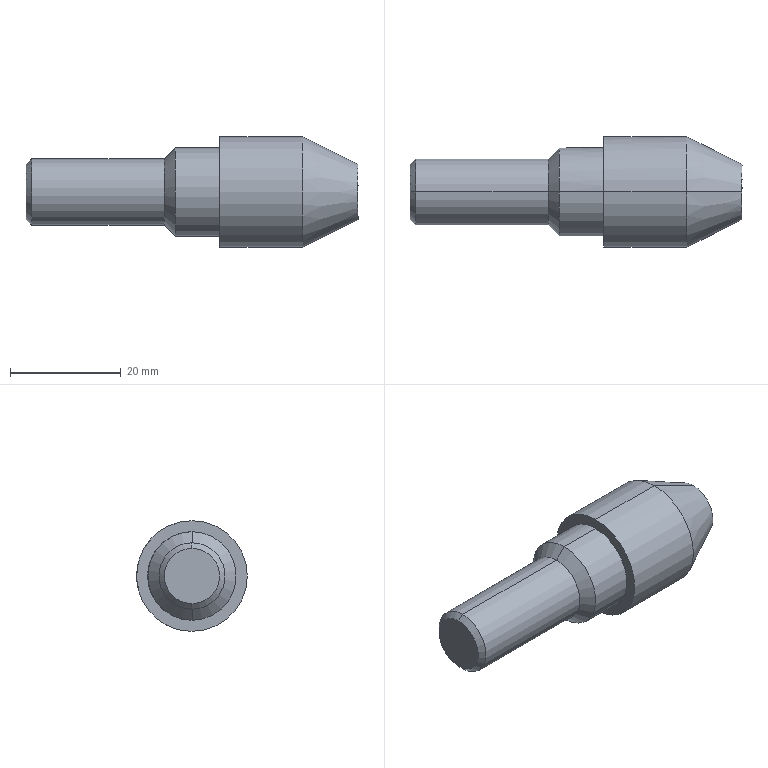Part | STEP file | Positioning_id698_x_t | 1 solid | 15 faces | box 60 x 20 x 20 mm | volume 11273 mm3 | cone 6 | cylinder 6 | plane 3 | commonest cylinder face diameters 12 x2 16 x2 20 x2
STEP:
#1=CARTESIAN_POINT('',(0.,0.,0.));
#2=DIRECTION('',(0.,0.,1.));
#3=DIRECTION('',(1.,0.,0.));
#4=AXIS2_PLACEMENT_3D('',#1,#2,#3);
#5=CARTESIAN_POINT('',(-988.002,780.,192.466));
#6=VERTEX_POINT('',#5);
#7=CARTESIAN_POINT('',(-998.002,780.,187.466));
#8=VERTEX_POINT('',#7);
#9=CARTESIAN_POINT('',(-988.002,780.,192.466));
#10=DIRECTION('',(-0.8944,0.,-0.4472));
#11=VECTOR('',#10,1.);
#12=LINE('',#9,#11);
#13=CARTESIAN_POINT('',(-998.002,780.,197.466));
#14=DIRECTION('',(-1.,0.,0.));
#15=DIRECTION('',(0.,0.,-1.));
#16=AXIS2_PLACEMENT_3D('',#13,#14,#15);
#17=CONICAL_SURFACE('',#16,10.,0.4636);
#18=CARTESIAN_POINT('',(0.,-10.));
#19=DIRECTION('',(0.,1.));
#20=VECTOR('',#19,1.);
#21=LINE('',#18,#20);
#22=(GEOMETRIC_REPRESENTATION_CONTEXT(2)PARAMETRIC_REPRESENTATION_CONTEXT()REPRESENTATION_CONTEXT('',''));
#23=DEFINITIONAL_REPRESENTATION('',(#21),#22);
#24=PCURVE('',#17,#23);
#25=CARTESIAN_POINT('',(-998.002,780.,197.466));
#26=DIRECTION('',(-1.,0.,0.));
#27=DIRECTION('',(0.,0.,-1.));
#28=AXIS2_PLACEMENT_3D('',#25,#26,#27);
#29=CONICAL_SURFACE('',#28,10.,0.4636);
#30=CARTESIAN_POINT('',(6.283,-10.));
#31=DIRECTION('',(0.,1.));
#32=VECTOR('',#31,1.);
#33=LINE('',#30,#32);
#34=(GEOMETRIC_REPRESENTATION_CONTEXT(2)PARAMETRIC_REPRESENTATION_CONTEXT()REPRESENTATION_CONTEXT('',''));
#35=DEFINITIONAL_REPRESENTATION('',(#33),#34);
#36=PCURVE('',#29,#35);
#37=SURFACE_CURVE('',#12,(#24,#36),.PCURVE_S1.);
#38=EDGE_CURVE('',#6,#8,#37,.T.);
#39=ORIENTED_EDGE('',*,*,#38,.F.);
#40=CARTESIAN_POINT('',(-988.002,780.,202.466));
#41=VERTEX_POINT('',#40);
#42=CARTESIAN_POINT('',(-988.002,780.,197.466));
#43=DIRECTION('',(-1.,0.,0.));
#44=DIRECTION('',(0.,-1.,0.));
#45=AXIS2_PLACEMENT_3D('',#42,#43,#44);
#46=CIRCLE('',#45,5.);
#47=CARTESIAN_POINT('',(-4.712,-10.));
#48=DIRECTION('',(1.,0.));
#49=VECTOR('',#48,1.);
#50=LINE('',#47,#49);
#51=(GEOMETRIC_REPRESENTATION_CONTEXT(2)PARAMETRIC_REPRESENTATION_CONTEXT()REPRESENTATION_CONTEXT('',''));
#52=DEFINITIONAL_REPRESENTATION('',(#50),#51);
#53=PCURVE('',#17,#52);
#54=CARTESIAN_POINT('',(-988.002,780.,197.466));
#55=DIRECTION('',(1.,0.,0.));
#56=DIRECTION('',(0.,0.,1.));
#57=AXIS2_PLACEMENT_3D('',#54,#55,#56);
#58=PLANE('',#57);
#59=CARTESIAN_POINT('',(0.,5.));
#60=CARTESIAN_POINT('',(8.66,5.));
#61=CARTESIAN_POINT('',(4.33,-2.5));
#62=CARTESIAN_POINT('',(0.,-10.));
#63=CARTESIAN_POINT('',(-4.33,-2.5));
#64=CARTESIAN_POINT('',(-8.66,5.));
#65=CARTESIAN_POINT('',(0.,5.));
#66=(BOUNDED_CURVE()B_SPLINE_CURVE(2,(#59,#60,#61,#62,#63,#64,#65),.UNSPECIFIED.,.T.,.F.)B_SPLINE_CURVE_WITH_KNOTS((1,2,2,2,2,1),(-2.094,0.,2.094,4.189,6.283,8.378),.UNSPECIFIED.)CURVE()GEOMETRIC_REPRESENTATION_ITEM()RATIONAL_B_SPLINE_CURVE((1.,0.5,1.,0.5,1.,0.5,1.))REPRESENTATION_ITEM(''));
#67=(GEOMETRIC_REPRESENTATION_CONTEXT(2)PARAMETRIC_REPRESENTATION_CONTEXT()REPRESENTATION_CONTEXT('',''));
#68=DEFINITIONAL_REPRESENTATION('',(#66),#67);
#69=PCURVE('',#58,#68);
#70=SURFACE_CURVE('',#46,(#53,#69),.PCURVE_S1.);
#71=EDGE_CURVE('',#6,#41,#70,.T.);
#72=ORIENTED_EDGE('',*,*,#71,.T.);
#73=CARTESIAN_POINT('',(-998.002,780.,207.466));
#74=VERTEX_POINT('',#73);
#75=CARTESIAN_POINT('',(-988.002,780.,202.466));
#76=DIRECTION('',(0.8944,0.,-0.4472));
#77=VECTOR('',#76,1.);
#78=LINE('',#75,#77);
#79=CARTESIAN_POINT('',(3.142,-10.));
#80=DIRECTION('',(0.,-1.));
#81=VECTOR('',#80,1.);
#82=LINE('',#79,#81);
#83=(GEOMETRIC_REPRESENTATION_CONTEXT(2)PARAMETRIC_REPRESENTATION_CONTEXT()REPRESENTATION_CONTEXT('',''));
#84=DEFINITIONAL_REPRESENTATION('',(#82),#83);
#85=PCURVE('',#17,#84);
#86=CARTESIAN_POINT('',(3.142,-10.));
#87=DIRECTION('',(0.,-1.));
#88=VECTOR('',#87,1.);
#89=LINE('',#86,#88);
#90=(GEOMETRIC_REPRESENTATION_CONTEXT(2)PARAMETRIC_REPRESENTATION_CONTEXT()REPRESENTATION_CONTEXT('',''));
#91=DEFINITIONAL_REPRESENTATION('',(#89),#90);
#92=PCURVE('',#29,#91);
#93=SURFACE_CURVE('',#78,(#85,#92),.PCURVE_S1.);
#94=EDGE_CURVE('',#74,#41,#93,.T.);
#95=ORIENTED_EDGE('',*,*,#94,.F.);
#96=CARTESIAN_POINT('',(-998.002,780.,197.466));
#97=DIRECTION('',(-1.,0.,0.));
#98=DIRECTION('',(0.,0.,-1.));
#99=AXIS2_PLACEMENT_3D('',#96,#97,#98);
#100=CIRCLE('',#99,10.);
#101=CARTESIAN_POINT('',(0.,0.));
#102=DIRECTION('',(1.,0.));
#103=VECTOR('',#102,1.);
#104=LINE('',#101,#103);
#105=(GEOMETRIC_REPRESENTATION_CONTEXT(2)PARAMETRIC_REPRESENTATION_CONTEXT()REPRESENTATION_CONTEXT('',''));
#106=DEFINITIONAL_REPRESENTATION('',(#104),#105);
#107=PCURVE('',#17,#106);
#108=CARTESIAN_POINT('',(-988.002,780.,197.466));
#109=DIRECTION('',(1.,0.,0.));
#110=DIRECTION('',(0.,0.,-1.));
#111=AXIS2_PLACEMENT_3D('',#108,#109,#110);
#112=CYLINDRICAL_SURFACE('',#111,10.);
#113=CARTESIAN_POINT('',(6.283,-10.));
#114=DIRECTION('',(-1.,0.));
#115=VECTOR('',#114,1.);
#116=LINE('',#113,#115);
#117=(GEOMETRIC_REPRESENTATION_CONTEXT(2)PARAMETRIC_REPRESENTATION_CONTEXT()REPRESENTATION_CONTEXT('',''));
#118=DEFINITIONAL_REPRESENTATION('',(#116),#117);
#119=PCURVE('',#112,#118);
#120=SURFACE_CURVE('',#100,(#107,#119),.PCURVE_S1.);
#121=EDGE_CURVE('',#8,#74,#120,.T.);
#122=ORIENTED_EDGE('',*,*,#121,.F.);
#123=EDGE_LOOP('',(#39,#72,#95,#122));
#124=FACE_BOUND('',#123,.T.);
#125=ADVANCED_FACE('',(#124),#17,.T.);
#126=CARTESIAN_POINT('',(-988.002,780.,202.466));
#127=CARTESIAN_POINT('',(-988.002,785.,202.466));
#128=CARTESIAN_POINT('',(-988.002,787.5,197.466));
#129=CARTESIAN_POINT('',(-988.002,785.,192.466));
#130=CARTESIAN_POINT('',(-988.002,780.,192.466));
#131=(BOUNDED_CURVE()B_SPLINE_CURVE(4,(#126,#127,#128,#129,#130),.UNSPECIFIED.,.F.,.F.)B_SPLINE_CURVE_WITH_KNOTS((5,5),(0.,1.),.PIECEWISE_BEZIER_KNOTS.)CURVE()GEOMETRIC_REPRESENTATION_ITEM()RATIONAL_B_SPLINE_CURVE((1.,0.7071,0.6667,0.7071,1.))REPRESENTATION_ITEM(''));
#132=CARTESIAN_POINT('',(5.,0.));
#133=CARTESIAN_POINT('',(5.,-5.));
#134=CARTESIAN_POINT('',(0.,-7.5));
#135=CARTESIAN_POINT('',(-5.,-5.));
#136=CARTESIAN_POINT('',(-5.,0.));
#137=(BOUNDED_CURVE()B_SPLINE_CURVE(4,(#132,#133,#134,#135,#136),.UNSPECIFIED.,.F.,.F.)B_SPLINE_CURVE_WITH_KNOTS((5,5),(0.,1.),.PIECEWISE_BEZIER_KNOTS.)CURVE()GEOMETRIC_REPRESENTATION_ITEM()RATIONAL_B_SPLINE_CURVE((1.,0.7071,0.6667,0.7071,1.))REPRESENTATION_ITEM(''));
#138=(GEOMETRIC_REPRESENTATION_CONTEXT(2)PARAMETRIC_REPRESENTATION_CONTEXT()REPRESENTATION_CONTEXT('',''));
#139=DEFINITIONAL_REPRESENTATION('',(#137),#138);
#140=PCURVE('',#58,#139);
#141=CARTESIAN_POINT('',(3.142,-10.));
#142=CARTESIAN_POINT('',(3.184,-10.));
#143=CARTESIAN_POINT('',(3.271,-10.));
#144=CARTESIAN_POINT('',(3.405,-10.));
#145=CARTESIAN_POINT('',(3.542,-10.));
#146=CARTESIAN_POINT('',(3.681,-10.));
#147=CARTESIAN_POINT('',(3.823,-10.));
#148=CARTESIAN_POINT('',(3.968,-10.));
#149=CARTESIAN_POINT('',(4.114,-10.));
#150=CARTESIAN_POINT('',(4.262,-10.));
#151=CARTESIAN_POINT('',(4.412,-10.));
#152=CARTESIAN_POINT('',(4.562,-10.));
#153=CARTESIAN_POINT('',(4.712,-10.));
#154=CARTESIAN_POINT('',(4.863,-10.));
#155=CARTESIAN_POINT('',(5.013,-10.));
#156=CARTESIAN_POINT('',(5.163,-10.));
#157=CARTESIAN_POINT('',(5.311,-10.));
#158=CARTESIAN_POINT('',(5.457,-10.));
#159=CARTESIAN_POINT('',(5.602,-10.));
#160=CARTESIAN_POINT('',(5.744,-10.));
#161=CARTESIAN_POINT('',(5.883,-10.));
#162=CARTESIAN_POINT('',(6.02,-10.));
#163=CARTESIAN_POINT('',(6.153,-10.));
#164=CARTESIAN_POINT('',(6.24,-10.));
#165=CARTESIAN_POINT('',(6.283,-10.));
#166=B_SPLINE_CURVE_WITH_KNOTS('',3,(#141,#142,#143,#144,#145,#146,#147,#148,#149,#150,#151,#152,#153,#154,#155,#156,#157,#158,#159,#160,#161,#162,#163,#164,#165),.UNSPECIFIED.,.F.,.F.,(4,1,1,1,1,1,1,1,1,1,1,1,1,1,1,1,1,1,1,1,1,1,4),(0.,0.04545,0.09091,0.1364,0.1818,0.2273,0.2727,0.3182,0.3636,0.4091,0.4545,0.5,0.5455,0.5909,0.6364,0.6818,0.7273,0.7727,0.8182,0.8636,0.9091,0.9545,1.),.QUASI_UNIFORM_KNOTS.);
#167=(GEOMETRIC_REPRESENTATION_CONTEXT(2)PARAMETRIC_REPRESENTATION_CONTEXT()REPRESENTATION_CONTEXT('',''));
#168=DEFINITIONAL_REPRESENTATION('',(#166),#167);
#169=PCURVE('',#29,#168);
#170=SURFACE_CURVE('',#131,(#140,#169),.PCURVE_S1.);
#171=EDGE_CURVE('',#41,#6,#170,.T.);
#172=ORIENTED_EDGE('',*,*,#171,.F.);
#173=ORIENTED_EDGE('',*,*,#71,.F.);
#174=EDGE_LOOP('',(#172,#173));
#175=FACE_BOUND('',#174,.T.);
#176=ADVANCED_FACE('',(#175),#58,.T.);
#177=CARTESIAN_POINT('',(-1047.002,780.,203.466));
#178=VERTEX_POINT('',#177);
#179=CARTESIAN_POINT('',(-1048.002,780.,202.466));
#180=VERTEX_POINT('',#179);
#181=CARTESIAN_POINT('',(-1048.002,780.,202.466));
#182=DIRECTION('',(-0.7071,0.,-0.7071));
#183=VECTOR('',#182,1.);
#184=LINE('',#181,#183);
#185=CARTESIAN_POINT('',(-1047.002,780.,197.466));
#186=DIRECTION('',(1.,0.,0.));
#187=DIRECTION('',(0.,0.,1.));
#188=AXIS2_PLACEMENT_3D('',#185,#186,#187);
#189=CONICAL_SURFACE('',#188,6.,0.7854);
#190=CARTESIAN_POINT('',(0.,-1.));
#191=DIRECTION('',(0.,-1.));
#192=VECTOR('',#191,1.);
#193=LINE('',#190,#192);
#194=(GEOMETRIC_REPRESENTATION_CONTEXT(2)PARAMETRIC_REPRESENTATION_CONTEXT()REPRESENTATION_CONTEXT('',''));
#195=DEFINITIONAL_REPRESENTATION('',(#193),#194);
#196=PCURVE('',#189,#195);
#197=CARTESIAN_POINT('',(-1047.002,780.,197.466));
#198=DIRECTION('',(1.,0.,0.));
#199=DIRECTION('',(0.,0.,1.));
#200=AXIS2_PLACEMENT_3D('',#197,#198,#199);
#201=CONICAL_SURFACE('',#200,6.,0.7854);
#202=CARTESIAN_POINT('',(6.283,-1.));
#203=DIRECTION('',(0.,-1.));
#204=VECTOR('',#203,1.);
#205=LINE('',#202,#204);
#206=(GEOMETRIC_REPRESENTATION_CONTEXT(2)PARAMETRIC_REPRESENTATION_CONTEXT()REPRESENTATION_CONTEXT('',''));
#207=DEFINITIONAL_REPRESENTATION('',(#205),#206);
#208=PCURVE('',#201,#207);
#209=SURFACE_CURVE('',#184,(#196,#208),.PCURVE_S1.);
#210=EDGE_CURVE('',#178,#180,#209,.T.);
#211=ORIENTED_EDGE('',*,*,#210,.T.);
#212=CARTESIAN_POINT('',(-1048.002,780.,192.466));
#213=VERTEX_POINT('',#212);
#214=CARTESIAN_POINT('',(-1048.002,780.,197.466));
#215=DIRECTION('',(1.,0.,0.));
#216=DIRECTION('',(0.,1.,0.));
#217=AXIS2_PLACEMENT_3D('',#214,#215,#216);
#218=CIRCLE('',#217,5.);
#219=CARTESIAN_POINT('',(-1.571,-1.));
#220=DIRECTION('',(1.,0.));
#221=VECTOR('',#220,1.);
#222=LINE('',#219,#221);
#223=(GEOMETRIC_REPRESENTATION_CONTEXT(2)PARAMETRIC_REPRESENTATION_CONTEXT()REPRESENTATION_CONTEXT('',''));
#224=DEFINITIONAL_REPRESENTATION('',(#222),#223);
#225=PCURVE('',#189,#224);
#226=CARTESIAN_POINT('',(-1048.002,780.,197.466));
#227=DIRECTION('',(-1.,0.,0.));
#228=DIRECTION('',(0.,0.,-1.));
#229=AXIS2_PLACEMENT_3D('',#226,#227,#228);
#230=PLANE('',#229);
#231=CARTESIAN_POINT('',(0.,-5.));
#232=CARTESIAN_POINT('',(-8.66,-5.));
#233=CARTESIAN_POINT('',(-4.33,2.5));
#234=CARTESIAN_POINT('',(0.,10.));
#235=CARTESIAN_POINT('',(4.33,2.5));
#236=CARTESIAN_POINT('',(8.66,-5.));
#237=CARTESIAN_POINT('',(0.,-5.));
#238=(BOUNDED_CURVE()B_SPLINE_CURVE(2,(#231,#232,#233,#234,#235,#236,#237),.UNSPECIFIED.,.T.,.F.)B_SPLINE_CURVE_WITH_KNOTS((1,2,2,2,2,1),(-2.094,0.,2.094,4.189,6.283,8.378),.UNSPECIFIED.)CURVE()GEOMETRIC_REPRESENTATION_ITEM()RATIONAL_B_SPLINE_CURVE((1.,0.5,1.,0.5,1.,0.5,1.))REPRESENTATION_ITEM(''));
#239=(GEOMETRIC_REPRESENTATION_CONTEXT(2)PARAMETRIC_REPRESENTATION_CONTEXT()REPRESENTATION_CONTEXT('',''));
#240=DEFINITIONAL_REPRESENTATION('',(#238),#239);
#241=PCURVE('',#230,#240);
#242=SURFACE_CURVE('',#218,(#225,#241),.PCURVE_S1.);
#243=EDGE_CURVE('',#180,#213,#242,.T.);
#244=ORIENTED_EDGE('',*,*,#243,.T.);
#245=CARTESIAN_POINT('',(-1047.002,780.,191.466));
#246=VERTEX_POINT('',#245);
#247=CARTESIAN_POINT('',(-1048.002,780.,192.466));
#248=DIRECTION('',(0.7071,0.,-0.7071));
#249=VECTOR('',#248,1.);
#250=LINE('',#247,#249);
#251=CARTESIAN_POINT('',(3.142,-1.));
#252=DIRECTION('',(0.,1.));
#253=VECTOR('',#252,1.);
#254=LINE('',#251,#253);
#255=(GEOMETRIC_REPRESENTATION_CONTEXT(2)PARAMETRIC_REPRESENTATION_CONTEXT()REPRESENTATION_CONTEXT('',''));
#256=DEFINITIONAL_REPRESENTATION('',(#254),#255);
#257=PCURVE('',#189,#256);
#258=CARTESIAN_POINT('',(3.142,-1.));
#259=DIRECTION('',(0.,1.));
#260=VECTOR('',#259,1.);
#261=LINE('',#258,#260);
#262=(GEOMETRIC_REPRESENTATION_CONTEXT(2)PARAMETRIC_REPRESENTATION_CONTEXT()REPRESENTATION_CONTEXT('',''));
#263=DEFINITIONAL_REPRESENTATION('',(#261),#262);
#264=PCURVE('',#201,#263);
#265=SURFACE_CURVE('',#250,(#257,#264),.PCURVE_S1.);
#266=EDGE_CURVE('',#213,#246,#265,.T.);
#267=ORIENTED_EDGE('',*,*,#266,.T.);
#268=CARTESIAN_POINT('',(-1047.002,780.,197.466));
#269=DIRECTION('',(-1.,0.,0.));
#270=DIRECTION('',(0.,0.,-1.));
#271=AXIS2_PLACEMENT_3D('',#268,#269,#270);
#272=CIRCLE('',#271,6.);
#273=CARTESIAN_POINT('',(3.142,0.));
#274=DIRECTION('',(-1.,0.));
#275=VECTOR('',#274,1.);
#276=LINE('',#273,#275);
#277=(GEOMETRIC_REPRESENTATION_CONTEXT(2)PARAMETRIC_REPRESENTATION_CONTEXT()REPRESENTATION_CONTEXT('',''));
#278=DEFINITIONAL_REPRESENTATION('',(#276),#277);
#279=PCURVE('',#189,#278);
#280=CARTESIAN_POINT('',(-1023.002,780.,197.466));
#281=DIRECTION('',(1.,0.,0.));
#282=DIRECTION('',(0.,0.,-1.));
#283=AXIS2_PLACEMENT_3D('',#280,#281,#282);
#284=CYLINDRICAL_SURFACE('',#283,6.);
#285=CARTESIAN_POINT('',(6.283,-24.));
#286=DIRECTION('',(-1.,0.));
#287=VECTOR('',#286,1.);
#288=LINE('',#285,#287);
#289=(GEOMETRIC_REPRESENTATION_CONTEXT(2)PARAMETRIC_REPRESENTATION_CONTEXT()REPRESENTATION_CONTEXT('',''));
#290=DEFINITIONAL_REPRESENTATION('',(#288),#289);
#291=PCURVE('',#284,#290);
#292=SURFACE_CURVE('',#272,(#279,#291),.PCURVE_S1.);
#293=EDGE_CURVE('',#246,#178,#292,.T.);
#294=ORIENTED_EDGE('',*,*,#293,.T.);
#295=EDGE_LOOP('',(#211,#244,#267,#294));
#296=FACE_BOUND('',#295,.T.);
#297=ADVANCED_FACE('',(#296),#189,.T.);
#298=CARTESIAN_POINT('',(-1023.002,780.,191.466));
#299=VERTEX_POINT('',#298);
#300=CARTESIAN_POINT('',(-1023.002,780.,191.466));
#301=DIRECTION('',(-1.,0.,0.));
#302=VECTOR('',#301,1.);
#303=LINE('',#300,#302);
#304=CARTESIAN_POINT('',(6.283,0.));
#305=DIRECTION('',(0.,-1.));
#306=VECTOR('',#305,1.);
#307=LINE('',#304,#306);
#308=(GEOMETRIC_REPRESENTATION_CONTEXT(2)PARAMETRIC_REPRESENTATION_CONTEXT()REPRESENTATION_CONTEXT('',''));
#309=DEFINITIONAL_REPRESENTATION('',(#307),#308);
#310=PCURVE('',#284,#309);
#311=CARTESIAN_POINT('',(-1023.002,780.,197.466));
#312=DIRECTION('',(1.,0.,0.));
#313=DIRECTION('',(0.,0.,-1.));
#314=AXIS2_PLACEMENT_3D('',#311,#312,#313);
#315=CYLINDRICAL_SURFACE('',#314,6.);
#316=CARTESIAN_POINT('',(0.,0.));
#317=DIRECTION('',(0.,-1.));
#318=VECTOR('',#317,1.);
#319=LINE('',#316,#318);
#320=(GEOMETRIC_REPRESENTATION_CONTEXT(2)PARAMETRIC_REPRESENTATION_CONTEXT()REPRESENTATION_CONTEXT('',''));
#321=DEFINITIONAL_REPRESENTATION('',(#319),#320);
#322=PCURVE('',#315,#321);
#323=SURFACE_CURVE('',#303,(#310,#322),.PCURVE_S1.);
#324=EDGE_CURVE('',#299,#246,#323,.T.);
#325=ORIENTED_EDGE('',*,*,#324,.F.);
#326=CARTESIAN_POINT('',(-1023.002,780.,203.466));
#327=VERTEX_POINT('',#326);
#328=CARTESIAN_POINT('',(-1023.002,780.,197.466));
#329=DIRECTION('',(1.,0.,0.));
#330=DIRECTION('',(0.,0.,1.));
#331=AXIS2_PLACEMENT_3D('',#328,#329,#330);
#332=CIRCLE('',#331,6.);
#333=CARTESIAN_POINT('',(3.142,0.));
#334=DIRECTION('',(1.,0.));
#335=VECTOR('',#334,1.);
#336=LINE('',#333,#335);
#337=(GEOMETRIC_REPRESENTATION_CONTEXT(2)PARAMETRIC_REPRESENTATION_CONTEXT()REPRESENTATION_CONTEXT('',''));
#338=DEFINITIONAL_REPRESENTATION('',(#336),#337);
#339=PCURVE('',#284,#338);
#340=CARTESIAN_POINT('',(-1021.002,780.,197.466));
#341=DIRECTION('',(1.,0.,0.));
#342=DIRECTION('',(0.,0.,1.));
#343=AXIS2_PLACEMENT_3D('',#340,#341,#342);
#344=CONICAL_SURFACE('',#343,8.,0.7854);
#345=CARTESIAN_POINT('',(0.,-2.));
#346=DIRECTION('',(1.,0.));
#347=VECTOR('',#346,1.);
#348=LINE('',#345,#347);
#349=(GEOMETRIC_REPRESENTATION_CONTEXT(2)PARAMETRIC_REPRESENTATION_CONTEXT()REPRESENTATION_CONTEXT('',''));
#350=DEFINITIONAL_REPRESENTATION('',(#348),#349);
#351=PCURVE('',#344,#350);
#352=SURFACE_CURVE('',#332,(#339,#351),.PCURVE_S1.);
#353=EDGE_CURVE('',#327,#299,#352,.T.);
#354=ORIENTED_EDGE('',*,*,#353,.F.);
#355=CARTESIAN_POINT('',(-1023.002,780.,203.466));
#356=DIRECTION('',(1.,0.,0.));
#357=VECTOR('',#356,1.);
#358=LINE('',#355,#357);
#359=CARTESIAN_POINT('',(3.142,0.));
#360=DIRECTION('',(0.,1.));
#361=VECTOR('',#360,1.);
#362=LINE('',#359,#361);
#363=(GEOMETRIC_REPRESENTATION_CONTEXT(2)PARAMETRIC_REPRESENTATION_CONTEXT()REPRESENTATION_CONTEXT('',''));
#364=DEFINITIONAL_REPRESENTATION('',(#362),#363);
#365=PCURVE('',#284,#364);
#366=CARTESIAN_POINT('',(3.142,0.));
#367=DIRECTION('',(0.,1.));
#368=VECTOR('',#367,1.);
#369=LINE('',#366,#368);
#370=(GEOMETRIC_REPRESENTATION_CONTEXT(2)PARAMETRIC_REPRESENTATION_CONTEXT()REPRESENTATION_CONTEXT('',''));
#371=DEFINITIONAL_REPRESENTATION('',(#369),#370);
#372=PCURVE('',#315,#371);
#373=SURFACE_CURVE('',#358,(#365,#372),.PCURVE_S1.);
#374=EDGE_CURVE('',#178,#327,#373,.T.);
#375=ORIENTED_EDGE('',*,*,#374,.F.);
#376=ORIENTED_EDGE('',*,*,#293,.F.);
#377=EDGE_LOOP('',(#325,#354,#375,#376));
#378=FACE_BOUND('',#377,.T.);
#379=ADVANCED_FACE('',(#378),#284,.T.);
#380=CARTESIAN_POINT('',(-1048.002,780.,192.466));
#381=CARTESIAN_POINT('',(-1048.002,785.,192.466));
#382=CARTESIAN_POINT('',(-1048.002,787.5,197.466));
#383=CARTESIAN_POINT('',(-1048.002,785.,202.466));
#384=CARTESIAN_POINT('',(-1048.002,780.,202.466));
#385=(BOUNDED_CURVE()B_SPLINE_CURVE(4,(#380,#381,#382,#383,#384),.UNSPECIFIED.,.F.,.F.)B_SPLINE_CURVE_WITH_KNOTS((5,5),(0.,1.),.PIECEWISE_BEZIER_KNOTS.)CURVE()GEOMETRIC_REPRESENTATION_ITEM()RATIONAL_B_SPLINE_CURVE((1.,0.7071,0.6667,0.7071,1.))REPRESENTATION_ITEM(''));
#386=CARTESIAN_POINT('',(5.,0.));
#387=CARTESIAN_POINT('',(5.,-5.));
#388=CARTESIAN_POINT('',(0.,-7.5));
#389=CARTESIAN_POINT('',(-5.,-5.));
#390=CARTESIAN_POINT('',(-5.,0.));
#391=(BOUNDED_CURVE()B_SPLINE_CURVE(4,(#386,#387,#388,#389,#390),.UNSPECIFIED.,.F.,.F.)B_SPLINE_CURVE_WITH_KNOTS((5,5),(0.,1.),.PIECEWISE_BEZIER_KNOTS.)CURVE()GEOMETRIC_REPRESENTATION_ITEM()RATIONAL_B_SPLINE_CURVE((1.,0.7071,0.6667,0.7071,1.))REPRESENTATION_ITEM(''));
#392=(GEOMETRIC_REPRESENTATION_CONTEXT(2)PARAMETRIC_REPRESENTATION_CONTEXT()REPRESENTATION_CONTEXT('',''));
#393=DEFINITIONAL_REPRESENTATION('',(#391),#392);
#394=PCURVE('',#230,#393);
#395=CARTESIAN_POINT('',(3.142,-1.));
#396=CARTESIAN_POINT('',(3.184,-1.));
#397=CARTESIAN_POINT('',(3.271,-1.));
#398=CARTESIAN_POINT('',(3.405,-1.));
#399=CARTESIAN_POINT('',(3.542,-1.));
#400=CARTESIAN_POINT('',(3.681,-1.));
#401=CARTESIAN_POINT('',(3.823,-1.));
#402=CARTESIAN_POINT('',(3.968,-1.));
#403=CARTESIAN_POINT('',(4.114,-1.));
#404=CARTESIAN_POINT('',(4.262,-1.));
#405=CARTESIAN_POINT('',(4.412,-1.));
#406=CARTESIAN_POINT('',(4.562,-1.));
#407=CARTESIAN_POINT('',(4.712,-1.));
#408=CARTESIAN_POINT('',(4.863,-1.));
#409=CARTESIAN_POINT('',(5.013,-1.));
#410=CARTESIAN_POINT('',(5.163,-1.));
#411=CARTESIAN_POINT('',(5.311,-1.));
#412=CARTESIAN_POINT('',(5.457,-1.));
#413=CARTESIAN_POINT('',(5.602,-1.));
#414=CARTESIAN_POINT('',(5.744,-1.));
#415=CARTESIAN_POINT('',(5.883,-1.));
#416=CARTESIAN_POINT('',(6.02,-1.));
#417=CARTESIAN_POINT('',(6.153,-1.));
#418=CARTESIAN_POINT('',(6.24,-1.));
#419=CARTESIAN_POINT('',(6.283,-1.));
#420=B_SPLINE_CURVE_WITH_KNOTS('',3,(#395,#396,#397,#398,#399,#400,#401,#402,#403,#404,#405,#406,#407,#408,#409,#410,#411,#412,#413,#414,#415,#416,#417,#418,#419),.UNSPECIFIED.,.F.,.F.,(4,1,1,1,1,1,1,1,1,1,1,1,1,1,1,1,1,1,1,1,1,1,4),(0.,0.04545,0.09091,0.1364,0.1818,0.2273,0.2727,0.3182,0.3636,0.4091,0.4545,0.5,0.5455,0.5909,0.6364,0.6818,0.7273,0.7727,0.8182,0.8636,0.9091,0.9545,1.),.QUASI_UNIFORM_KNOTS.);
#421=(GEOMETRIC_REPRESENTATION_CONTEXT(2)PARAMETRIC_REPRESENTATION_CONTEXT()REPRESENTATION_CONTEXT('',''));
#422=DEFINITIONAL_REPRESENTATION('',(#420),#421);
#423=PCURVE('',#201,#422);
#424=SURFACE_CURVE('',#385,(#394,#423),.PCURVE_S1.);
#425=EDGE_CURVE('',#213,#180,#424,.T.);
#426=ORIENTED_EDGE('',*,*,#425,.F.);
#427=ORIENTED_EDGE('',*,*,#243,.F.);
#428=EDGE_LOOP('',(#426,#427));
#429=FACE_BOUND('',#428,.T.);
#430=ADVANCED_FACE('',(#429),#230,.T.);
#431=CARTESIAN_POINT('',(-1021.002,780.,205.466));
#432=VERTEX_POINT('',#431);
#433=CARTESIAN_POINT('',(-1023.002,780.,203.466));
#434=DIRECTION('',(0.7071,0.,0.7071));
#435=VECTOR('',#434,1.);
#436=LINE('',#433,#435);
#437=CARTESIAN_POINT('',(0.,-2.));
#438=DIRECTION('',(0.,1.));
#439=VECTOR('',#438,1.);
#440=LINE('',#437,#439);
#441=(GEOMETRIC_REPRESENTATION_CONTEXT(2)PARAMETRIC_REPRESENTATION_CONTEXT()REPRESENTATION_CONTEXT('',''));
#442=DEFINITIONAL_REPRESENTATION('',(#440),#441);
#443=PCURVE('',#344,#442);
#444=CARTESIAN_POINT('',(-1021.002,780.,197.466));
#445=DIRECTION('',(1.,0.,0.));
#446=DIRECTION('',(0.,0.,1.));
#447=AXIS2_PLACEMENT_3D('',#444,#445,#446);
#448=CONICAL_SURFACE('',#447,8.,0.7854);
#449=CARTESIAN_POINT('',(6.283,-2.));
#450=DIRECTION('',(0.,1.));
#451=VECTOR('',#450,1.);
#452=LINE('',#449,#451);
#453=(GEOMETRIC_REPRESENTATION_CONTEXT(2)PARAMETRIC_REPRESENTATION_CONTEXT()REPRESENTATION_CONTEXT('',''));
#454=DEFINITIONAL_REPRESENTATION('',(#452),#453);
#455=PCURVE('',#448,#454);
#456=SURFACE_CURVE('',#436,(#443,#455),.PCURVE_S1.);
#457=EDGE_CURVE('',#327,#432,#456,.T.);
#458=ORIENTED_EDGE('',*,*,#457,.F.);
#459=ORIENTED_EDGE('',*,*,#353,.T.);
#460=CARTESIAN_POINT('',(-1021.002,780.,189.466));
#461=VERTEX_POINT('',#460);
#462=CARTESIAN_POINT('',(-1023.002,780.,191.466));
#463=DIRECTION('',(-0.7071,0.,0.7071));
#464=VECTOR('',#463,1.);
#465=LINE('',#462,#464);
#466=CARTESIAN_POINT('',(3.142,-2.));
#467=DIRECTION('',(0.,-1.));
#468=VECTOR('',#467,1.);
#469=LINE('',#466,#468);
#470=(GEOMETRIC_REPRESENTATION_CONTEXT(2)PARAMETRIC_REPRESENTATION_CONTEXT()REPRESENTATION_CONTEXT('',''));
#471=DEFINITIONAL_REPRESENTATION('',(#469),#470);
#472=PCURVE('',#344,#471);
#473=CARTESIAN_POINT('',(3.142,-2.));
#474=DIRECTION('',(0.,-1.));
#475=VECTOR('',#474,1.);
#476=LINE('',#473,#475);
#477=(GEOMETRIC_REPRESENTATION_CONTEXT(2)PARAMETRIC_REPRESENTATION_CONTEXT()REPRESENTATION_CONTEXT('',''));
#478=DEFINITIONAL_REPRESENTATION('',(#476),#477);
#479=PCURVE('',#448,#478);
#480=SURFACE_CURVE('',#465,(#472,#479),.PCURVE_S1.);
#481=EDGE_CURVE('',#461,#299,#480,.T.);
#482=ORIENTED_EDGE('',*,*,#481,.F.);
#483=CARTESIAN_POINT('',(-1021.002,780.,197.466));
#484=DIRECTION('',(-1.,0.,0.));
#485=DIRECTION('',(0.,0.,-1.));
#486=AXIS2_PLACEMENT_3D('',#483,#484,#485);
#487=CIRCLE('',#486,8.);
#488=CARTESIAN_POINT('',(3.142,0.));
#489=DIRECTION('',(-1.,0.));
#490=VECTOR('',#489,1.);
#491=LINE('',#488,#490);
#492=(GEOMETRIC_REPRESENTATION_CONTEXT(2)PARAMETRIC_REPRESENTATION_CONTEXT()REPRESENTATION_CONTEXT('',''));
#493=DEFINITIONAL_REPRESENTATION('',(#491),#492);
#494=PCURVE('',#344,#493);
#495=CARTESIAN_POINT('',(-1013.002,780.,197.466));
#496=DIRECTION('',(1.,0.,0.));
#497=DIRECTION('',(0.,0.,-1.));
#498=AXIS2_PLACEMENT_3D('',#495,#496,#497);
#499=CYLINDRICAL_SURFACE('',#498,8.);
#500=CARTESIAN_POINT('',(6.283,-8.));
#501=DIRECTION('',(-1.,0.));
#502=VECTOR('',#501,1.);
#503=LINE('',#500,#502);
#504=(GEOMETRIC_REPRESENTATION_CONTEXT(2)PARAMETRIC_REPRESENTATION_CONTEXT()REPRESENTATION_CONTEXT('',''));
#505=DEFINITIONAL_REPRESENTATION('',(#503),#504);
#506=PCURVE('',#499,#505);
#507=SURFACE_CURVE('',#487,(#494,#506),.PCURVE_S1.);
#508=EDGE_CURVE('',#461,#432,#507,.T.);
#509=ORIENTED_EDGE('',*,*,#508,.T.);
#510=EDGE_LOOP('',(#458,#459,#482,#509));
#511=FACE_BOUND('',#510,.T.);
#512=ADVANCED_FACE('',(#511),#344,.T.);
#513=CARTESIAN_POINT('',(-1013.002,780.,189.466));
#514=VERTEX_POINT('',#513);
#515=CARTESIAN_POINT('',(-1013.002,780.,189.466));
#516=DIRECTION('',(1.,0.,0.));
#517=VECTOR('',#516,1.);
#518=LINE('',#515,#517);
#519=CARTESIAN_POINT('',(6.283,0.));
#520=DIRECTION('',(0.,1.));
#521=VECTOR('',#520,1.);
#522=LINE('',#519,#521);
#523=(GEOMETRIC_REPRESENTATION_CONTEXT(2)PARAMETRIC_REPRESENTATION_CONTEXT()REPRESENTATION_CONTEXT('',''));
#524=DEFINITIONAL_REPRESENTATION('',(#522),#523);
#525=PCURVE('',#499,#524);
#526=CARTESIAN_POINT('',(-1013.002,780.,197.466));
#527=DIRECTION('',(1.,0.,0.));
#528=DIRECTION('',(0.,0.,-1.));
#529=AXIS2_PLACEMENT_3D('',#526,#527,#528);
#530=CYLINDRICAL_SURFACE('',#529,8.);
#531=CARTESIAN_POINT('',(0.,0.));
#532=DIRECTION('',(0.,1.));
#533=VECTOR('',#532,1.);
#534=LINE('',#531,#533);
#535=(GEOMETRIC_REPRESENTATION_CONTEXT(2)PARAMETRIC_REPRESENTATION_CONTEXT()REPRESENTATION_CONTEXT('',''));
#536=DEFINITIONAL_REPRESENTATION('',(#534),#535);
#537=PCURVE('',#530,#536);
#538=SURFACE_CURVE('',#518,(#525,#537),.PCURVE_S1.);
#539=EDGE_CURVE('',#461,#514,#538,.T.);
#540=ORIENTED_EDGE('',*,*,#539,.T.);
#541=CARTESIAN_POINT('',(-1013.002,780.,205.466));
#542=VERTEX_POINT('',#541);
#543=CARTESIAN_POINT('',(-1013.002,780.,197.466));
#544=DIRECTION('',(1.,0.,0.));
#545=DIRECTION('',(0.,0.,-1.));
#546=AXIS2_PLACEMENT_3D('',#543,#544,#545);
#547=CIRCLE('',#546,8.);
#548=CARTESIAN_POINT('',(0.,0.));
#549=DIRECTION('',(1.,0.));
#550=VECTOR('',#549,1.);
#551=LINE('',#548,#550);
#552=(GEOMETRIC_REPRESENTATION_CONTEXT(2)PARAMETRIC_REPRESENTATION_CONTEXT()REPRESENTATION_CONTEXT('',''));
#553=DEFINITIONAL_REPRESENTATION('',(#551),#552);
#554=PCURVE('',#499,#553);
#555=CARTESIAN_POINT('',(-1013.002,780.,197.466));
#556=DIRECTION('',(-1.,0.,0.));
#557=DIRECTION('',(0.,0.,-1.));
#558=AXIS2_PLACEMENT_3D('',#555,#556,#557);
#559=PLANE('',#558);
#560=CARTESIAN_POINT('',(8.,0.));
#561=CARTESIAN_POINT('',(8.,-13.856));
#562=CARTESIAN_POINT('',(-4.,-6.928));
#563=CARTESIAN_POINT('',(-16.,0.));
#564=CARTESIAN_POINT('',(-4.,6.928));
#565=CARTESIAN_POINT('',(8.,13.856));
#566=CARTESIAN_POINT('',(8.,0.));
#567=(BOUNDED_CURVE()B_SPLINE_CURVE(2,(#560,#561,#562,#563,#564,#565,#566),.UNSPECIFIED.,.T.,.F.)B_SPLINE_CURVE_WITH_KNOTS((1,2,2,2,2,1),(-2.094,0.,2.094,4.189,6.283,8.378),.UNSPECIFIED.)CURVE()GEOMETRIC_REPRESENTATION_ITEM()RATIONAL_B_SPLINE_CURVE((1.,0.5,1.,0.5,1.,0.5,1.))REPRESENTATION_ITEM(''));
#568=(GEOMETRIC_REPRESENTATION_CONTEXT(2)PARAMETRIC_REPRESENTATION_CONTEXT()REPRESENTATION_CONTEXT('',''));
#569=DEFINITIONAL_REPRESENTATION('',(#567),#568);
#570=PCURVE('',#559,#569);
#571=SURFACE_CURVE('',#547,(#554,#570),.PCURVE_S1.);
#572=EDGE_CURVE('',#542,#514,#571,.T.);
#573=ORIENTED_EDGE('',*,*,#572,.F.);
#574=CARTESIAN_POINT('',(-1013.002,780.,205.466));
#575=DIRECTION('',(-1.,0.,0.));
#576=VECTOR('',#575,1.);
#577=LINE('',#574,#576);
#578=CARTESIAN_POINT('',(3.142,0.));
#579=DIRECTION('',(0.,-1.));
#580=VECTOR('',#579,1.);
#581=LINE('',#578,#580);
#582=(GEOMETRIC_REPRESENTATION_CONTEXT(2)PARAMETRIC_REPRESENTATION_CONTEXT()REPRESENTATION_CONTEXT('',''));
#583=DEFINITIONAL_REPRESENTATION('',(#581),#582);
#584=PCURVE('',#499,#583);
#585=CARTESIAN_POINT('',(3.142,0.));
#586=DIRECTION('',(0.,-1.));
#587=VECTOR('',#586,1.);
#588=LINE('',#585,#587);
#589=(GEOMETRIC_REPRESENTATION_CONTEXT(2)PARAMETRIC_REPRESENTATION_CONTEXT()REPRESENTATION_CONTEXT('',''));
#590=DEFINITIONAL_REPRESENTATION('',(#588),#589);
#591=PCURVE('',#530,#590);
#592=SURFACE_CURVE('',#577,(#584,#591),.PCURVE_S1.);
#593=EDGE_CURVE('',#542,#432,#592,.T.);
#594=ORIENTED_EDGE('',*,*,#593,.T.);
#595=ORIENTED_EDGE('',*,*,#508,.F.);
#596=EDGE_LOOP('',(#540,#573,#594,#595));
#597=FACE_BOUND('',#596,.T.);
#598=ADVANCED_FACE('',(#597),#499,.T.);
#599=CARTESIAN_POINT('',(-1013.002,780.,187.466));
#600=VERTEX_POINT('',#599);
#601=CARTESIAN_POINT('',(-998.002,780.,187.466));
#602=DIRECTION('',(-1.,0.,0.));
#603=VECTOR('',#602,1.);
#604=LINE('',#601,#603);
#605=CARTESIAN_POINT('',(6.283,-10.));
#606=DIRECTION('',(0.,-1.));
#607=VECTOR('',#606,1.);
#608=LINE('',#605,#607);
#609=(GEOMETRIC_REPRESENTATION_CONTEXT(2)PARAMETRIC_REPRESENTATION_CONTEXT()REPRESENTATION_CONTEXT('',''));
#610=DEFINITIONAL_REPRESENTATION('',(#608),#609);
#611=PCURVE('',#112,#610);
#612=CARTESIAN_POINT('',(-988.002,780.,197.466));
#613=DIRECTION('',(1.,0.,0.));
#614=DIRECTION('',(0.,0.,-1.));
#615=AXIS2_PLACEMENT_3D('',#612,#613,#614);
#616=CYLINDRICAL_SURFACE('',#615,10.);
#617=CARTESIAN_POINT('',(0.,-10.));
#618=DIRECTION('',(0.,-1.));
#619=VECTOR('',#618,1.);
#620=LINE('',#617,#619);
#621=(GEOMETRIC_REPRESENTATION_CONTEXT(2)PARAMETRIC_REPRESENTATION_CONTEXT()REPRESENTATION_CONTEXT('',''));
#622=DEFINITIONAL_REPRESENTATION('',(#620),#621);
#623=PCURVE('',#616,#622);
#624=SURFACE_CURVE('',#604,(#611,#623),.PCURVE_S1.);
#625=EDGE_CURVE('',#8,#600,#624,.T.);
#626=ORIENTED_EDGE('',*,*,#625,.F.);
#627=ORIENTED_EDGE('',*,*,#121,.T.);
#628=CARTESIAN_POINT('',(-1013.002,780.,207.466));
#629=VERTEX_POINT('',#628);
#630=CARTESIAN_POINT('',(-998.002,780.,207.466));
#631=DIRECTION('',(1.,0.,0.));
#632=VECTOR('',#631,1.);
#633=LINE('',#630,#632);
#634=CARTESIAN_POINT('',(3.142,-10.));
#635=DIRECTION('',(0.,1.));
#636=VECTOR('',#635,1.);
#637=LINE('',#634,#636);
#638=(GEOMETRIC_REPRESENTATION_CONTEXT(2)PARAMETRIC_REPRESENTATION_CONTEXT()REPRESENTATION_CONTEXT('',''));
#639=DEFINITIONAL_REPRESENTATION('',(#637),#638);
#640=PCURVE('',#112,#639);
#641=CARTESIAN_POINT('',(3.142,-10.));
#642=DIRECTION('',(0.,1.));
#643=VECTOR('',#642,1.);
#644=LINE('',#641,#643);
#645=(GEOMETRIC_REPRESENTATION_CONTEXT(2)PARAMETRIC_REPRESENTATION_CONTEXT()REPRESENTATION_CONTEXT('',''));
#646=DEFINITIONAL_REPRESENTATION('',(#644),#645);
#647=PCURVE('',#616,#646);
#648=SURFACE_CURVE('',#633,(#640,#647),.PCURVE_S1.);
#649=EDGE_CURVE('',#629,#74,#648,.T.);
#650=ORIENTED_EDGE('',*,*,#649,.F.);
#651=CARTESIAN_POINT('',(-1013.002,780.,197.466));
#652=DIRECTION('',(-1.,0.,0.));
#653=DIRECTION('',(0.,1.,0.));
#654=AXIS2_PLACEMENT_3D('',#651,#652,#653);
#655=CIRCLE('',#654,10.);
#656=CARTESIAN_POINT('',(7.854,-25.));
#657=DIRECTION('',(-1.,0.));
#658=VECTOR('',#657,1.);
#659=LINE('',#656,#658);
#660=(GEOMETRIC_REPRESENTATION_CONTEXT(2)PARAMETRIC_REPRESENTATION_CONTEXT()REPRESENTATION_CONTEXT('',''));
#661=DEFINITIONAL_REPRESENTATION('',(#659),#660);
#662=PCURVE('',#112,#661);
#663=CARTESIAN_POINT('',(0.,0.));
#664=DIRECTION('',(0.,-1.));
#665=AXIS2_PLACEMENT_2D('',#663,#664);
#666=CIRCLE('',#665,10.);
#667=(GEOMETRIC_REPRESENTATION_CONTEXT(2)PARAMETRIC_REPRESENTATION_CONTEXT()REPRESENTATION_CONTEXT('',''));
#668=DEFINITIONAL_REPRESENTATION('',(#666),#667);
#669=PCURVE('',#559,#668);
#670=SURFACE_CURVE('',#655,(#662,#669),.PCURVE_S1.);
#671=EDGE_CURVE('',#600,#629,#670,.T.);
#672=ORIENTED_EDGE('',*,*,#671,.F.);
#673=EDGE_LOOP('',(#626,#627,#650,#672));
#674=FACE_BOUND('',#673,.T.);
#675=ADVANCED_FACE('',(#674),#112,.T.);
#676=ORIENTED_EDGE('',*,*,#572,.T.);
#677=CARTESIAN_POINT('',(-1013.002,780.,189.466));
#678=CARTESIAN_POINT('',(-1013.002,788.,189.466));
#679=CARTESIAN_POINT('',(-1013.002,792.,197.466));
#680=CARTESIAN_POINT('',(-1013.002,788.,205.466));
#681=CARTESIAN_POINT('',(-1013.002,780.,205.466));
#682=(BOUNDED_CURVE()B_SPLINE_CURVE(4,(#677,#678,#679,#680,#681),.UNSPECIFIED.,.F.,.F.)B_SPLINE_CURVE_WITH_KNOTS((5,5),(0.,1.),.PIECEWISE_BEZIER_KNOTS.)CURVE()GEOMETRIC_REPRESENTATION_ITEM()RATIONAL_B_SPLINE_CURVE((1.,0.7071,0.6667,0.7071,1.))REPRESENTATION_ITEM(''));
#683=CARTESIAN_POINT('',(8.,0.));
#684=CARTESIAN_POINT('',(8.,-8.));
#685=CARTESIAN_POINT('',(0.,-12.));
#686=CARTESIAN_POINT('',(-8.,-8.));
#687=CARTESIAN_POINT('',(-8.,0.));
#688=(BOUNDED_CURVE()B_SPLINE_CURVE(4,(#683,#684,#685,#686,#687),.UNSPECIFIED.,.F.,.F.)B_SPLINE_CURVE_WITH_KNOTS((5,5),(0.,1.),.PIECEWISE_BEZIER_KNOTS.)CURVE()GEOMETRIC_REPRESENTATION_ITEM()RATIONAL_B_SPLINE_CURVE((1.,0.7071,0.6667,0.7071,1.))REPRESENTATION_ITEM(''));
#689=(GEOMETRIC_REPRESENTATION_CONTEXT(2)PARAMETRIC_REPRESENTATION_CONTEXT()REPRESENTATION_CONTEXT('',''));
#690=DEFINITIONAL_REPRESENTATION('',(#688),#689);
#691=PCURVE('',#559,#690);
#692=CARTESIAN_POINT('',(0.,0.));
#693=CARTESIAN_POINT('',(0.04285,0.));
#694=CARTESIAN_POINT('',(0.1297,0.));
#695=CARTESIAN_POINT('',(0.2633,0.));
#696=CARTESIAN_POINT('',(0.3999,0.));
#697=CARTESIAN_POINT('',(0.5394,0.));
#698=CARTESIAN_POINT('',(0.6816,0.));
#699=CARTESIAN_POINT('',(0.8261,0.));
#700=CARTESIAN_POINT('',(0.9725,0.));
#701=CARTESIAN_POINT('',(1.121,0.));
#702=CARTESIAN_POINT('',(1.27,0.));
#703=CARTESIAN_POINT('',(1.42,0.));
#704=CARTESIAN_POINT('',(1.571,0.));
#705=CARTESIAN_POINT('',(1.721,0.));
#706=CARTESIAN_POINT('',(1.872,0.));
#707=CARTESIAN_POINT('',(2.021,0.));
#708=CARTESIAN_POINT('',(2.169,0.));
#709=CARTESIAN_POINT('',(2.316,0.));
#710=CARTESIAN_POINT('',(2.46,0.));
#711=CARTESIAN_POINT('',(2.602,0.));
#712=CARTESIAN_POINT('',(2.742,0.));
#713=CARTESIAN_POINT('',(2.878,0.));
#714=CARTESIAN_POINT('',(3.012,0.));
#715=CARTESIAN_POINT('',(3.099,0.));
#716=CARTESIAN_POINT('',(3.142,0.));
#717=B_SPLINE_CURVE_WITH_KNOTS('',3,(#692,#693,#694,#695,#696,#697,#698,#699,#700,#701,#702,#703,#704,#705,#706,#707,#708,#709,#710,#711,#712,#713,#714,#715,#716),.UNSPECIFIED.,.F.,.F.,(4,1,1,1,1,1,1,1,1,1,1,1,1,1,1,1,1,1,1,1,1,1,4),(0.,0.04545,0.09091,0.1364,0.1818,0.2273,0.2727,0.3182,0.3636,0.4091,0.4545,0.5,0.5455,0.5909,0.6364,0.6818,0.7273,0.7727,0.8182,0.8636,0.9091,0.9545,1.),.QUASI_UNIFORM_KNOTS.);
#718=(GEOMETRIC_REPRESENTATION_CONTEXT(2)PARAMETRIC_REPRESENTATION_CONTEXT()REPRESENTATION_CONTEXT('',''));
#719=DEFINITIONAL_REPRESENTATION('',(#717),#718);
#720=PCURVE('',#530,#719);
#721=SURFACE_CURVE('',#682,(#691,#720),.PCURVE_S1.);
#722=EDGE_CURVE('',#514,#542,#721,.T.);
#723=ORIENTED_EDGE('',*,*,#722,.T.);
#724=EDGE_LOOP('',(#676,#723));
#725=FACE_BOUND('',#724,.T.);
#726=CARTESIAN_POINT('',(-1013.002,780.,207.466));
#727=CARTESIAN_POINT('',(-1013.002,790.,207.466));
#728=CARTESIAN_POINT('',(-1013.002,795.,197.466));
#729=CARTESIAN_POINT('',(-1013.002,790.,187.466));
#730=CARTESIAN_POINT('',(-1013.002,780.,187.466));
#731=(BOUNDED_CURVE()B_SPLINE_CURVE(4,(#726,#727,#728,#729,#730),.UNSPECIFIED.,.F.,.F.)B_SPLINE_CURVE_WITH_KNOTS((5,5),(0.,1.),.PIECEWISE_BEZIER_KNOTS.)CURVE()GEOMETRIC_REPRESENTATION_ITEM()RATIONAL_B_SPLINE_CURVE((1.,0.7071,0.6667,0.7071,1.))REPRESENTATION_ITEM(''));
#732=CARTESIAN_POINT('',(-10.,0.));
#733=CARTESIAN_POINT('',(-10.,-10.));
#734=CARTESIAN_POINT('',(0.,-15.));
#735=CARTESIAN_POINT('',(10.,-10.));
#736=CARTESIAN_POINT('',(10.,0.));
#737=(BOUNDED_CURVE()B_SPLINE_CURVE(4,(#732,#733,#734,#735,#736),.UNSPECIFIED.,.F.,.F.)B_SPLINE_CURVE_WITH_KNOTS((5,5),(0.,1.),.PIECEWISE_BEZIER_KNOTS.)CURVE()GEOMETRIC_REPRESENTATION_ITEM()RATIONAL_B_SPLINE_CURVE((1.,0.7071,0.6667,0.7071,1.))REPRESENTATION_ITEM(''));
#738=(GEOMETRIC_REPRESENTATION_CONTEXT(2)PARAMETRIC_REPRESENTATION_CONTEXT()REPRESENTATION_CONTEXT('',''));
#739=DEFINITIONAL_REPRESENTATION('',(#737),#738);
#740=PCURVE('',#559,#739);
#741=CARTESIAN_POINT('',(3.142,-25.));
#742=CARTESIAN_POINT('',(3.099,-25.));
#743=CARTESIAN_POINT('',(3.012,-25.));
#744=CARTESIAN_POINT('',(2.878,-25.));
#745=CARTESIAN_POINT('',(2.742,-25.));
#746=CARTESIAN_POINT('',(2.602,-25.));
#747=CARTESIAN_POINT('',(2.46,-25.));
#748=CARTESIAN_POINT('',(2.316,-25.));
#749=CARTESIAN_POINT('',(2.169,-25.));
#750=CARTESIAN_POINT('',(2.021,-25.));
#751=CARTESIAN_POINT('',(1.872,-25.));
#752=CARTESIAN_POINT('',(1.721,-25.));
#753=CARTESIAN_POINT('',(1.571,-25.));
#754=CARTESIAN_POINT('',(1.42,-25.));
#755=CARTESIAN_POINT('',(1.27,-25.));
#756=CARTESIAN_POINT('',(1.121,-25.));
#757=CARTESIAN_POINT('',(0.9725,-25.));
#758=CARTESIAN_POINT('',(0.8261,-25.));
#759=CARTESIAN_POINT('',(0.6816,-25.));
#760=CARTESIAN_POINT('',(0.5394,-25.));
#761=CARTESIAN_POINT('',(0.3999,-25.));
#762=CARTESIAN_POINT('',(0.2633,-25.));
#763=CARTESIAN_POINT('',(0.1297,-25.));
#764=CARTESIAN_POINT('',(0.04285,-25.));
#765=CARTESIAN_POINT('',(0.,-25.));
#766=B_SPLINE_CURVE_WITH_KNOTS('',3,(#741,#742,#743,#744,#745,#746,#747,#748,#749,#750,#751,#752,#753,#754,#755,#756,#757,#758,#759,#760,#761,#762,#763,#764,#765),.UNSPECIFIED.,.F.,.F.,(4,1,1,1,1,1,1,1,1,1,1,1,1,1,1,1,1,1,1,1,1,1,4),(0.,0.04545,0.09091,0.1364,0.1818,0.2273,0.2727,0.3182,0.3636,0.4091,0.4545,0.5,0.5455,0.5909,0.6364,0.6818,0.7273,0.7727,0.8182,0.8636,0.9091,0.9545,1.),.QUASI_UNIFORM_KNOTS.);
#767=(GEOMETRIC_REPRESENTATION_CONTEXT(2)PARAMETRIC_REPRESENTATION_CONTEXT()REPRESENTATION_CONTEXT('',''));
#768=DEFINITIONAL_REPRESENTATION('',(#766),#767);
#769=PCURVE('',#616,#768);
#770=SURFACE_CURVE('',#731,(#740,#769),.PCURVE_S1.);
#771=EDGE_CURVE('',#629,#600,#770,.T.);
#772=ORIENTED_EDGE('',*,*,#771,.T.);
#773=ORIENTED_EDGE('',*,*,#671,.T.);
#774=EDGE_LOOP('',(#772,#773));
#775=FACE_BOUND('',#774,.T.);
#776=ADVANCED_FACE('',(#725,#775),#559,.T.);
#777=CARTESIAN_POINT('',(-998.002,780.,197.466));
#778=DIRECTION('',(-1.,0.,0.));
#779=DIRECTION('',(0.,0.,1.));
#780=AXIS2_PLACEMENT_3D('',#777,#778,#779);
#781=CIRCLE('',#780,10.);
#782=CARTESIAN_POINT('',(3.142,-10.));
#783=DIRECTION('',(-1.,0.));
#784=VECTOR('',#783,1.);
#785=LINE('',#782,#784);
#786=(GEOMETRIC_REPRESENTATION_CONTEXT(2)PARAMETRIC_REPRESENTATION_CONTEXT()REPRESENTATION_CONTEXT('',''));
#787=DEFINITIONAL_REPRESENTATION('',(#785),#786);
#788=PCURVE('',#616,#787);
#789=CARTESIAN_POINT('',(3.142,0.));
#790=DIRECTION('',(1.,0.));
#791=VECTOR('',#790,1.);
#792=LINE('',#789,#791);
#793=(GEOMETRIC_REPRESENTATION_CONTEXT(2)PARAMETRIC_REPRESENTATION_CONTEXT()REPRESENTATION_CONTEXT('',''));
#794=DEFINITIONAL_REPRESENTATION('',(#792),#793);
#795=PCURVE('',#29,#794);
#796=SURFACE_CURVE('',#781,(#788,#795),.PCURVE_S1.);
#797=EDGE_CURVE('',#74,#8,#796,.T.);
#798=ORIENTED_EDGE('',*,*,#797,.T.);
#799=ORIENTED_EDGE('',*,*,#625,.T.);
#800=ORIENTED_EDGE('',*,*,#771,.F.);
#801=ORIENTED_EDGE('',*,*,#649,.T.);
#802=EDGE_LOOP('',(#798,#799,#800,#801));
#803=FACE_BOUND('',#802,.T.);
#804=ADVANCED_FACE('',(#803),#616,.T.);
#805=ORIENTED_EDGE('',*,*,#722,.F.);
#806=ORIENTED_EDGE('',*,*,#539,.F.);
#807=CARTESIAN_POINT('',(-1021.002,780.,197.466));
#808=DIRECTION('',(-1.,0.,0.));
#809=DIRECTION('',(0.,0.,1.));
#810=AXIS2_PLACEMENT_3D('',#807,#808,#809);
#811=CIRCLE('',#810,8.);
#812=CARTESIAN_POINT('',(3.142,-8.));
#813=DIRECTION('',(-1.,0.));
#814=VECTOR('',#813,1.);
#815=LINE('',#812,#814);
#816=(GEOMETRIC_REPRESENTATION_CONTEXT(2)PARAMETRIC_REPRESENTATION_CONTEXT()REPRESENTATION_CONTEXT('',''));
#817=DEFINITIONAL_REPRESENTATION('',(#815),#816);
#818=PCURVE('',#530,#817);
#819=CARTESIAN_POINT('',(6.283,0.));
#820=DIRECTION('',(-1.,0.));
#821=VECTOR('',#820,1.);
#822=LINE('',#819,#821);
#823=(GEOMETRIC_REPRESENTATION_CONTEXT(2)PARAMETRIC_REPRESENTATION_CONTEXT()REPRESENTATION_CONTEXT('',''));
#824=DEFINITIONAL_REPRESENTATION('',(#822),#823);
#825=PCURVE('',#448,#824);
#826=SURFACE_CURVE('',#811,(#818,#825),.PCURVE_S1.);
#827=EDGE_CURVE('',#432,#461,#826,.T.);
#828=ORIENTED_EDGE('',*,*,#827,.F.);
#829=ORIENTED_EDGE('',*,*,#593,.F.);
#830=EDGE_LOOP('',(#805,#806,#828,#829));
#831=FACE_BOUND('',#830,.T.);
#832=ADVANCED_FACE('',(#831),#530,.T.);
#833=CARTESIAN_POINT('',(-1023.002,780.,197.466));
#834=DIRECTION('',(1.,0.,0.));
#835=DIRECTION('',(0.,0.,-1.));
#836=AXIS2_PLACEMENT_3D('',#833,#834,#835);
#837=CIRCLE('',#836,6.);
#838=CARTESIAN_POINT('',(3.142,-2.));
#839=DIRECTION('',(1.,0.));
#840=VECTOR('',#839,1.);
#841=LINE('',#838,#840);
#842=(GEOMETRIC_REPRESENTATION_CONTEXT(2)PARAMETRIC_REPRESENTATION_CONTEXT()REPRESENTATION_CONTEXT('',''));
#843=DEFINITIONAL_REPRESENTATION('',(#841),#842);
#844=PCURVE('',#448,#843);
#845=CARTESIAN_POINT('',(0.,0.));
#846=DIRECTION('',(1.,0.));
#847=VECTOR('',#846,1.);
#848=LINE('',#845,#847);
#849=(GEOMETRIC_REPRESENTATION_CONTEXT(2)PARAMETRIC_REPRESENTATION_CONTEXT()REPRESENTATION_CONTEXT('',''));
#850=DEFINITIONAL_REPRESENTATION('',(#848),#849);
#851=PCURVE('',#315,#850);
#852=SURFACE_CURVE('',#837,(#844,#851),.PCURVE_S1.);
#853=EDGE_CURVE('',#299,#327,#852,.T.);
#854=ORIENTED_EDGE('',*,*,#853,.T.);
#855=ORIENTED_EDGE('',*,*,#457,.T.);
#856=ORIENTED_EDGE('',*,*,#827,.T.);
#857=ORIENTED_EDGE('',*,*,#481,.T.);
#858=EDGE_LOOP('',(#854,#855,#856,#857));
#859=FACE_BOUND('',#858,.T.);
#860=ADVANCED_FACE('',(#859),#448,.T.);
#861=ORIENTED_EDGE('',*,*,#853,.F.);
#862=ORIENTED_EDGE('',*,*,#324,.T.);
#863=CARTESIAN_POINT('',(-1047.002,780.,197.466));
#864=DIRECTION('',(-1.,0.,0.));
#865=DIRECTION('',(0.,0.,1.));
#866=AXIS2_PLACEMENT_3D('',#863,#864,#865);
#867=CIRCLE('',#866,6.);
#868=CARTESIAN_POINT('',(3.142,-24.));
#869=DIRECTION('',(-1.,0.));
#870=VECTOR('',#869,1.);
#871=LINE('',#868,#870);
#872=(GEOMETRIC_REPRESENTATION_CONTEXT(2)PARAMETRIC_REPRESENTATION_CONTEXT()REPRESENTATION_CONTEXT('',''));
#873=DEFINITIONAL_REPRESENTATION('',(#871),#872);
#874=PCURVE('',#315,#873);
#875=CARTESIAN_POINT('',(6.283,0.));
#876=DIRECTION('',(-1.,0.));
#877=VECTOR('',#876,1.);
#878=LINE('',#875,#877);
#879=(GEOMETRIC_REPRESENTATION_CONTEXT(2)PARAMETRIC_REPRESENTATION_CONTEXT()REPRESENTATION_CONTEXT('',''));
#880=DEFINITIONAL_REPRESENTATION('',(#878),#879);
#881=PCURVE('',#201,#880);
#882=SURFACE_CURVE('',#867,(#874,#881),.PCURVE_S1.);
#883=EDGE_CURVE('',#178,#246,#882,.T.);
#884=ORIENTED_EDGE('',*,*,#883,.F.);
#885=ORIENTED_EDGE('',*,*,#374,.T.);
#886=EDGE_LOOP('',(#861,#862,#884,#885));
#887=FACE_BOUND('',#886,.T.);
#888=ADVANCED_FACE('',(#887),#315,.T.);
#889=ORIENTED_EDGE('',*,*,#425,.T.);
#890=ORIENTED_EDGE('',*,*,#210,.F.);
#891=ORIENTED_EDGE('',*,*,#883,.T.);
#892=ORIENTED_EDGE('',*,*,#266,.F.);
#893=EDGE_LOOP('',(#889,#890,#891,#892));
#894=FACE_BOUND('',#893,.T.);
#895=ADVANCED_FACE('',(#894),#201,.T.);
#896=ORIENTED_EDGE('',*,*,#171,.T.);
#897=ORIENTED_EDGE('',*,*,#38,.T.);
#898=ORIENTED_EDGE('',*,*,#797,.F.);
#899=ORIENTED_EDGE('',*,*,#94,.T.);
#900=EDGE_LOOP('',(#896,#897,#898,#899));
#901=FACE_BOUND('',#900,.T.);
#902=ADVANCED_FACE('',(#901),#29,.T.);
#903=CLOSED_SHELL('',(#125,#176,#297,#379,#430,#512,#598,#675,#776,#804,#832,#860,#888,#895,#902));
#904=MANIFOLD_SOLID_BREP('',#903);
#905=(LENGTH_UNIT()NAMED_UNIT(*)SI_UNIT(.MILLI.,.METRE.));
#906=UNCERTAINTY_MEASURE_WITH_UNIT(LENGTH_MEASURE(0.0000001),#905,'','');
#907=(NAMED_UNIT(*)PLANE_ANGLE_UNIT()SI_UNIT($,.RADIAN.));
#908=(NAMED_UNIT(*)SI_UNIT($,.STERADIAN.)SOLID_ANGLE_UNIT());
#909=(GEOMETRIC_REPRESENTATION_CONTEXT(3)GLOBAL_UNCERTAINTY_ASSIGNED_CONTEXT((#906))GLOBAL_UNIT_ASSIGNED_CONTEXT((#905,#907,#908))REPRESENTATION_CONTEXT('',''));
#910=ADVANCED_BREP_SHAPE_REPRESENTATION('',(#4,#904),#909);